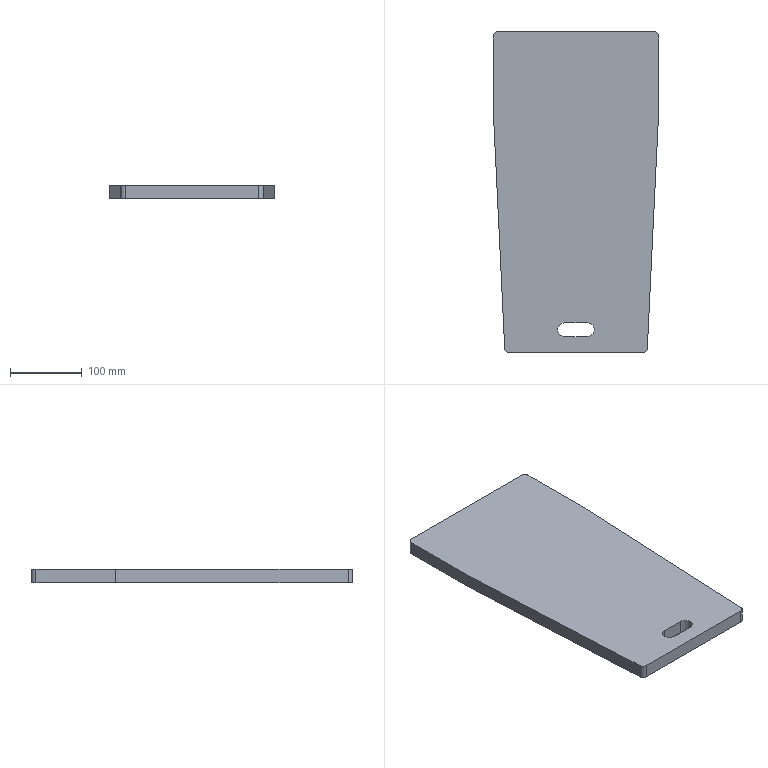Part | SolidWorks | features Extrusion 1 | 1 solid | 17 faces | box 230 x 447.55 x 19.05 mm | volume 1843027 mm3 | plane 10 | cylinder 7 | commonest cylinder face diameters 12.7 x4 19.05 x3
STEP:
#1=CARTESIAN_POINT('',(-15.875,9.525,9.525));
#2=VERTEX_POINT('',#1);
#3=CARTESIAN_POINT('',(-25.4,0.,9.525));
#4=VERTEX_POINT('',#3);
#5=CARTESIAN_POINT('',(-15.875,0.,9.525));
#6=DIRECTION('',(0.,0.,1.));
#7=DIRECTION('',(1.,0.,0.));
#8=AXIS2_PLACEMENT_3D('',#5,#6,#7);
#9=CIRCLE('',#8,9.525);
#10=EDGE_CURVE('',#2,#4,#9,.T.);
#11=ORIENTED_EDGE('',*,*,#10,.T.);
#12=CARTESIAN_POINT('',(-25.4,0.,-9.525));
#13=VERTEX_POINT('',#12);
#14=CARTESIAN_POINT('',(-25.4,0.,9.525));
#15=DIRECTION('',(0.,0.,-1.));
#16=VECTOR('',#15,1000.);
#17=LINE('',#14,#16);
#18=EDGE_CURVE('',#4,#13,#17,.T.);
#19=ORIENTED_EDGE('',*,*,#18,.T.);
#20=CARTESIAN_POINT('',(-15.875,9.525,-9.525));
#21=VERTEX_POINT('',#20);
#22=CARTESIAN_POINT('',(-15.875,0.,-9.525));
#23=DIRECTION('',(0.,0.,1.));
#24=DIRECTION('',(1.,0.,0.));
#25=AXIS2_PLACEMENT_3D('',#22,#23,#24);
#26=CIRCLE('',#25,9.525);
#27=EDGE_CURVE('',#21,#13,#26,.T.);
#28=ORIENTED_EDGE('',*,*,#27,.F.);
#29=CARTESIAN_POINT('',(-15.875,9.525,9.525));
#30=DIRECTION('',(0.,0.,-1.));
#31=VECTOR('',#30,1000.);
#32=LINE('',#29,#31);
#33=EDGE_CURVE('',#2,#21,#32,.T.);
#34=ORIENTED_EDGE('',*,*,#33,.F.);
#35=EDGE_LOOP('',(#11,#19,#28,#34));
#36=FACE_OUTER_BOUND('',#35,.T.);
#37=CARTESIAN_POINT('',(-15.875,0.,9.525));
#38=DIRECTION('',(0.,0.,-1.));
#39=DIRECTION('',(-1.,0.,0.));
#40=AXIS2_PLACEMENT_3D('',#37,#38,#39);
#41=CYLINDRICAL_SURFACE('',#40,9.525);
#42=ADVANCED_FACE('',(#36),#41,.F.);
#43=CARTESIAN_POINT('',(-115.,298.68,9.525));
#44=VERTEX_POINT('',#43);
#45=CARTESIAN_POINT('',(-99.352,-25.706,9.525));
#46=VERTEX_POINT('',#45);
#47=CARTESIAN_POINT('',(-115.,298.68,9.525));
#48=DIRECTION('',(0.04818,-0.9988,0.));
#49=VECTOR('',#48,1000.);
#50=LINE('',#47,#49);
#51=EDGE_CURVE('',#44,#46,#50,.T.);
#52=ORIENTED_EDGE('',*,*,#51,.T.);
#53=CARTESIAN_POINT('',(-93.009,-31.75,9.525));
#54=VERTEX_POINT('',#53);
#55=CARTESIAN_POINT('',(-93.009,-25.4,9.525));
#56=DIRECTION('',(0.,0.,1.));
#57=DIRECTION('',(1.,0.,0.));
#58=AXIS2_PLACEMENT_3D('',#55,#56,#57);
#59=CIRCLE('',#58,6.35);
#60=EDGE_CURVE('',#46,#54,#59,.T.);
#61=ORIENTED_EDGE('',*,*,#60,.T.);
#62=CARTESIAN_POINT('',(93.009,-31.75,9.525));
#63=VERTEX_POINT('',#62);
#64=CARTESIAN_POINT('',(-93.009,-31.75,9.525));
#65=DIRECTION('',(1.,0.,0.));
#66=VECTOR('',#65,1000.);
#67=LINE('',#64,#66);
#68=EDGE_CURVE('',#54,#63,#67,.T.);
#69=ORIENTED_EDGE('',*,*,#68,.T.);
#70=CARTESIAN_POINT('',(99.352,-25.706,9.525));
#71=VERTEX_POINT('',#70);
#72=CARTESIAN_POINT('',(93.009,-25.4,9.525));
#73=DIRECTION('',(0.,0.,1.));
#74=DIRECTION('',(-1.,0.,0.));
#75=AXIS2_PLACEMENT_3D('',#72,#73,#74);
#76=CIRCLE('',#75,6.35);
#77=EDGE_CURVE('',#63,#71,#76,.T.);
#78=ORIENTED_EDGE('',*,*,#77,.T.);
#79=CARTESIAN_POINT('',(115.,298.68,9.525));
#80=VERTEX_POINT('',#79);
#81=CARTESIAN_POINT('',(115.,298.68,9.525));
#82=DIRECTION('',(0.04818,0.9988,0.));
#83=VECTOR('',#82,1000.);
#84=LINE('',#81,#83);
#85=EDGE_CURVE('',#71,#80,#84,.T.);
#86=ORIENTED_EDGE('',*,*,#85,.T.);
#87=CARTESIAN_POINT('',(115.,409.45,9.525));
#88=VERTEX_POINT('',#87);
#89=CARTESIAN_POINT('',(115.,409.45,9.525));
#90=DIRECTION('',(0.,1.,0.));
#91=VECTOR('',#90,1000.);
#92=LINE('',#89,#91);
#93=EDGE_CURVE('',#80,#88,#92,.T.);
#94=ORIENTED_EDGE('',*,*,#93,.T.);
#95=CARTESIAN_POINT('',(108.65,415.8,9.525));
#96=VERTEX_POINT('',#95);
#97=CARTESIAN_POINT('',(108.65,409.45,9.525));
#98=DIRECTION('',(0.,0.,1.));
#99=DIRECTION('',(-1.,0.,0.));
#100=AXIS2_PLACEMENT_3D('',#97,#98,#99);
#101=CIRCLE('',#100,6.35);
#102=EDGE_CURVE('',#88,#96,#101,.T.);
#103=ORIENTED_EDGE('',*,*,#102,.T.);
#104=CARTESIAN_POINT('',(-108.65,415.8,9.525));
#105=VERTEX_POINT('',#104);
#106=CARTESIAN_POINT('',(108.65,415.8,9.525));
#107=DIRECTION('',(-1.,0.,0.));
#108=VECTOR('',#107,1000.);
#109=LINE('',#106,#108);
#110=EDGE_CURVE('',#96,#105,#109,.T.);
#111=ORIENTED_EDGE('',*,*,#110,.T.);
#112=CARTESIAN_POINT('',(-115.,409.45,9.525));
#113=VERTEX_POINT('',#112);
#114=CARTESIAN_POINT('',(-108.65,409.45,9.525));
#115=DIRECTION('',(0.,0.,1.));
#116=DIRECTION('',(1.,0.,0.));
#117=AXIS2_PLACEMENT_3D('',#114,#115,#116);
#118=CIRCLE('',#117,6.35);
#119=EDGE_CURVE('',#105,#113,#118,.T.);
#120=ORIENTED_EDGE('',*,*,#119,.T.);
#121=CARTESIAN_POINT('',(-115.,409.45,9.525));
#122=DIRECTION('',(0.,-1.,0.));
#123=VECTOR('',#122,1000.);
#124=LINE('',#121,#123);
#125=EDGE_CURVE('',#113,#44,#124,.T.);
#126=ORIENTED_EDGE('',*,*,#125,.T.);
#127=EDGE_LOOP('',(#52,#61,#69,#78,#86,#94,#103,#111,#120,#126));
#128=FACE_OUTER_BOUND('',#127,.T.);
#129=CARTESIAN_POINT('',(-15.875,-9.525,9.525));
#130=VERTEX_POINT('',#129);
#131=CARTESIAN_POINT('',(15.875,-9.525,9.525));
#132=VERTEX_POINT('',#131);
#133=CARTESIAN_POINT('',(-15.875,-9.525,9.525));
#134=DIRECTION('',(1.,0.,0.));
#135=VECTOR('',#134,1000.);
#136=LINE('',#133,#135);
#137=EDGE_CURVE('',#130,#132,#136,.T.);
#138=ORIENTED_EDGE('',*,*,#137,.F.);
#139=CARTESIAN_POINT('',(-15.875,0.,9.525));
#140=DIRECTION('',(0.,0.,1.));
#141=DIRECTION('',(1.,0.,0.));
#142=AXIS2_PLACEMENT_3D('',#139,#140,#141);
#143=CIRCLE('',#142,9.525);
#144=EDGE_CURVE('',#4,#130,#143,.T.);
#145=ORIENTED_EDGE('',*,*,#144,.F.);
#146=ORIENTED_EDGE('',*,*,#10,.F.);
#147=CARTESIAN_POINT('',(15.875,9.525,9.525));
#148=VERTEX_POINT('',#147);
#149=CARTESIAN_POINT('',(-15.875,9.525,9.525));
#150=DIRECTION('',(-1.,0.,0.));
#151=VECTOR('',#150,1000.);
#152=LINE('',#149,#151);
#153=EDGE_CURVE('',#148,#2,#152,.T.);
#154=ORIENTED_EDGE('',*,*,#153,.F.);
#155=CARTESIAN_POINT('',(15.875,0.,9.525));
#156=DIRECTION('',(0.,0.,1.));
#157=DIRECTION('',(1.,0.,0.));
#158=AXIS2_PLACEMENT_3D('',#155,#156,#157);
#159=CIRCLE('',#158,9.525);
#160=EDGE_CURVE('',#132,#148,#159,.T.);
#161=ORIENTED_EDGE('',*,*,#160,.F.);
#162=EDGE_LOOP('',(#138,#145,#146,#154,#161));
#163=FACE_BOUND('',#162,.T.);
#164=CARTESIAN_POINT('',(-93.009,-25.4,9.525));
#165=DIRECTION('',(0.,0.,1.));
#166=DIRECTION('',(1.,0.,0.));
#167=AXIS2_PLACEMENT_3D('',#164,#165,#166);
#168=PLANE('',#167);
#169=ADVANCED_FACE('',(#128,#163),#168,.T.);
#170=CARTESIAN_POINT('',(-115.,298.68,-9.525));
#171=VERTEX_POINT('',#170);
#172=CARTESIAN_POINT('',(-99.352,-25.706,-9.525));
#173=VERTEX_POINT('',#172);
#174=CARTESIAN_POINT('',(-115.,298.68,-9.525));
#175=DIRECTION('',(0.04818,-0.9988,0.));
#176=VECTOR('',#175,1000.);
#177=LINE('',#174,#176);
#178=EDGE_CURVE('',#171,#173,#177,.T.);
#179=ORIENTED_EDGE('',*,*,#178,.F.);
#180=CARTESIAN_POINT('',(-115.,409.45,-9.525));
#181=VERTEX_POINT('',#180);
#182=CARTESIAN_POINT('',(-115.,409.45,-9.525));
#183=DIRECTION('',(0.,-1.,0.));
#184=VECTOR('',#183,1000.);
#185=LINE('',#182,#184);
#186=EDGE_CURVE('',#181,#171,#185,.T.);
#187=ORIENTED_EDGE('',*,*,#186,.F.);
#188=CARTESIAN_POINT('',(-108.65,415.8,-9.525));
#189=VERTEX_POINT('',#188);
#190=CARTESIAN_POINT('',(-108.65,409.45,-9.525));
#191=DIRECTION('',(0.,0.,1.));
#192=DIRECTION('',(1.,0.,0.));
#193=AXIS2_PLACEMENT_3D('',#190,#191,#192);
#194=CIRCLE('',#193,6.35);
#195=EDGE_CURVE('',#189,#181,#194,.T.);
#196=ORIENTED_EDGE('',*,*,#195,.F.);
#197=CARTESIAN_POINT('',(108.65,415.8,-9.525));
#198=VERTEX_POINT('',#197);
#199=CARTESIAN_POINT('',(108.65,415.8,-9.525));
#200=DIRECTION('',(-1.,0.,0.));
#201=VECTOR('',#200,1000.);
#202=LINE('',#199,#201);
#203=EDGE_CURVE('',#198,#189,#202,.T.);
#204=ORIENTED_EDGE('',*,*,#203,.F.);
#205=CARTESIAN_POINT('',(115.,409.45,-9.525));
#206=VERTEX_POINT('',#205);
#207=CARTESIAN_POINT('',(108.65,409.45,-9.525));
#208=DIRECTION('',(0.,0.,1.));
#209=DIRECTION('',(-1.,0.,0.));
#210=AXIS2_PLACEMENT_3D('',#207,#208,#209);
#211=CIRCLE('',#210,6.35);
#212=EDGE_CURVE('',#206,#198,#211,.T.);
#213=ORIENTED_EDGE('',*,*,#212,.F.);
#214=CARTESIAN_POINT('',(115.,298.68,-9.525));
#215=VERTEX_POINT('',#214);
#216=CARTESIAN_POINT('',(115.,409.45,-9.525));
#217=DIRECTION('',(0.,1.,0.));
#218=VECTOR('',#217,1000.);
#219=LINE('',#216,#218);
#220=EDGE_CURVE('',#215,#206,#219,.T.);
#221=ORIENTED_EDGE('',*,*,#220,.F.);
#222=CARTESIAN_POINT('',(99.352,-25.706,-9.525));
#223=VERTEX_POINT('',#222);
#224=CARTESIAN_POINT('',(115.,298.68,-9.525));
#225=DIRECTION('',(0.04818,0.9988,0.));
#226=VECTOR('',#225,1000.);
#227=LINE('',#224,#226);
#228=EDGE_CURVE('',#223,#215,#227,.T.);
#229=ORIENTED_EDGE('',*,*,#228,.F.);
#230=CARTESIAN_POINT('',(93.009,-31.75,-9.525));
#231=VERTEX_POINT('',#230);
#232=CARTESIAN_POINT('',(93.009,-25.4,-9.525));
#233=DIRECTION('',(0.,0.,1.));
#234=DIRECTION('',(-1.,0.,0.));
#235=AXIS2_PLACEMENT_3D('',#232,#233,#234);
#236=CIRCLE('',#235,6.35);
#237=EDGE_CURVE('',#231,#223,#236,.T.);
#238=ORIENTED_EDGE('',*,*,#237,.F.);
#239=CARTESIAN_POINT('',(-93.009,-31.75,-9.525));
#240=VERTEX_POINT('',#239);
#241=CARTESIAN_POINT('',(-93.009,-31.75,-9.525));
#242=DIRECTION('',(1.,0.,0.));
#243=VECTOR('',#242,1000.);
#244=LINE('',#241,#243);
#245=EDGE_CURVE('',#240,#231,#244,.T.);
#246=ORIENTED_EDGE('',*,*,#245,.F.);
#247=CARTESIAN_POINT('',(-93.009,-25.4,-9.525));
#248=DIRECTION('',(0.,0.,1.));
#249=DIRECTION('',(1.,0.,0.));
#250=AXIS2_PLACEMENT_3D('',#247,#248,#249);
#251=CIRCLE('',#250,6.35);
#252=EDGE_CURVE('',#173,#240,#251,.T.);
#253=ORIENTED_EDGE('',*,*,#252,.F.);
#254=EDGE_LOOP('',(#179,#187,#196,#204,#213,#221,#229,#238,#246,#253));
#255=FACE_OUTER_BOUND('',#254,.T.);
#256=ORIENTED_EDGE('',*,*,#27,.T.);
#257=CARTESIAN_POINT('',(-15.875,-9.525,-9.525));
#258=VERTEX_POINT('',#257);
#259=CARTESIAN_POINT('',(-15.875,0.,-9.525));
#260=DIRECTION('',(0.,0.,1.));
#261=DIRECTION('',(1.,0.,0.));
#262=AXIS2_PLACEMENT_3D('',#259,#260,#261);
#263=CIRCLE('',#262,9.525);
#264=EDGE_CURVE('',#13,#258,#263,.T.);
#265=ORIENTED_EDGE('',*,*,#264,.T.);
#266=CARTESIAN_POINT('',(15.875,-9.525,-9.525));
#267=VERTEX_POINT('',#266);
#268=CARTESIAN_POINT('',(-15.875,-9.525,-9.525));
#269=DIRECTION('',(1.,0.,0.));
#270=VECTOR('',#269,1000.);
#271=LINE('',#268,#270);
#272=EDGE_CURVE('',#258,#267,#271,.T.);
#273=ORIENTED_EDGE('',*,*,#272,.T.);
#274=CARTESIAN_POINT('',(15.875,9.525,-9.525));
#275=VERTEX_POINT('',#274);
#276=CARTESIAN_POINT('',(15.875,0.,-9.525));
#277=DIRECTION('',(0.,0.,1.));
#278=DIRECTION('',(1.,0.,0.));
#279=AXIS2_PLACEMENT_3D('',#276,#277,#278);
#280=CIRCLE('',#279,9.525);
#281=EDGE_CURVE('',#267,#275,#280,.T.);
#282=ORIENTED_EDGE('',*,*,#281,.T.);
#283=CARTESIAN_POINT('',(-15.875,9.525,-9.525));
#284=DIRECTION('',(-1.,0.,0.));
#285=VECTOR('',#284,1000.);
#286=LINE('',#283,#285);
#287=EDGE_CURVE('',#275,#21,#286,.T.);
#288=ORIENTED_EDGE('',*,*,#287,.T.);
#289=EDGE_LOOP('',(#256,#265,#273,#282,#288));
#290=FACE_BOUND('',#289,.T.);
#291=CARTESIAN_POINT('',(-93.009,-25.4,-9.525));
#292=DIRECTION('',(0.,0.,1.));
#293=DIRECTION('',(1.,0.,0.));
#294=AXIS2_PLACEMENT_3D('',#291,#292,#293);
#295=PLANE('',#294);
#296=ADVANCED_FACE('',(#255,#290),#295,.F.);
#297=ORIENTED_EDGE('',*,*,#178,.T.);
#298=CARTESIAN_POINT('',(-99.352,-25.706,9.525));
#299=DIRECTION('',(0.,0.,-1.));
#300=VECTOR('',#299,1000.);
#301=LINE('',#298,#300);
#302=EDGE_CURVE('',#46,#173,#301,.T.);
#303=ORIENTED_EDGE('',*,*,#302,.F.);
#304=ORIENTED_EDGE('',*,*,#51,.F.);
#305=CARTESIAN_POINT('',(-115.,298.68,9.525));
#306=DIRECTION('',(0.,0.,-1.));
#307=VECTOR('',#306,1000.);
#308=LINE('',#305,#307);
#309=EDGE_CURVE('',#44,#171,#308,.T.);
#310=ORIENTED_EDGE('',*,*,#309,.T.);
#311=EDGE_LOOP('',(#297,#303,#304,#310));
#312=FACE_OUTER_BOUND('',#311,.T.);
#313=CARTESIAN_POINT('',(-115.,298.68,9.525));
#314=DIRECTION('',(0.9988,0.04818,0.));
#315=DIRECTION('',(-0.04818,0.9988,0.));
#316=AXIS2_PLACEMENT_3D('',#313,#314,#315);
#317=PLANE('',#316);
#318=ADVANCED_FACE('',(#312),#317,.F.);
#319=ORIENTED_EDGE('',*,*,#252,.T.);
#320=CARTESIAN_POINT('',(-93.009,-31.75,9.525));
#321=DIRECTION('',(0.,0.,-1.));
#322=VECTOR('',#321,1000.);
#323=LINE('',#320,#322);
#324=EDGE_CURVE('',#54,#240,#323,.T.);
#325=ORIENTED_EDGE('',*,*,#324,.F.);
#326=ORIENTED_EDGE('',*,*,#60,.F.);
#327=ORIENTED_EDGE('',*,*,#302,.T.);
#328=EDGE_LOOP('',(#319,#325,#326,#327));
#329=FACE_OUTER_BOUND('',#328,.T.);
#330=CARTESIAN_POINT('',(-93.009,-25.4,9.525));
#331=DIRECTION('',(0.,0.,-1.));
#332=DIRECTION('',(-1.,0.,0.));
#333=AXIS2_PLACEMENT_3D('',#330,#331,#332);
#334=CYLINDRICAL_SURFACE('',#333,6.35);
#335=ADVANCED_FACE('',(#329),#334,.T.);
#336=ORIENTED_EDGE('',*,*,#245,.T.);
#337=CARTESIAN_POINT('',(93.009,-31.75,9.525));
#338=DIRECTION('',(0.,0.,-1.));
#339=VECTOR('',#338,1000.);
#340=LINE('',#337,#339);
#341=EDGE_CURVE('',#63,#231,#340,.T.);
#342=ORIENTED_EDGE('',*,*,#341,.F.);
#343=ORIENTED_EDGE('',*,*,#68,.F.);
#344=ORIENTED_EDGE('',*,*,#324,.T.);
#345=EDGE_LOOP('',(#336,#342,#343,#344));
#346=FACE_OUTER_BOUND('',#345,.T.);
#347=CARTESIAN_POINT('',(-93.009,-31.75,9.525));
#348=DIRECTION('',(0.,1.,0.));
#349=DIRECTION('',(0.,0.,1.));
#350=AXIS2_PLACEMENT_3D('',#347,#348,#349);
#351=PLANE('',#350);
#352=ADVANCED_FACE('',(#346),#351,.F.);
#353=ORIENTED_EDGE('',*,*,#237,.T.);
#354=CARTESIAN_POINT('',(99.352,-25.706,9.525));
#355=DIRECTION('',(0.,0.,-1.));
#356=VECTOR('',#355,1000.);
#357=LINE('',#354,#356);
#358=EDGE_CURVE('',#71,#223,#357,.T.);
#359=ORIENTED_EDGE('',*,*,#358,.F.);
#360=ORIENTED_EDGE('',*,*,#77,.F.);
#361=ORIENTED_EDGE('',*,*,#341,.T.);
#362=EDGE_LOOP('',(#353,#359,#360,#361));
#363=FACE_OUTER_BOUND('',#362,.T.);
#364=CARTESIAN_POINT('',(93.009,-25.4,9.525));
#365=DIRECTION('',(0.,0.,-1.));
#366=DIRECTION('',(-1.,0.,0.));
#367=AXIS2_PLACEMENT_3D('',#364,#365,#366);
#368=CYLINDRICAL_SURFACE('',#367,6.35);
#369=ADVANCED_FACE('',(#363),#368,.T.);
#370=ORIENTED_EDGE('',*,*,#228,.T.);
#371=CARTESIAN_POINT('',(115.,298.68,9.525));
#372=DIRECTION('',(0.,0.,-1.));
#373=VECTOR('',#372,1000.);
#374=LINE('',#371,#373);
#375=EDGE_CURVE('',#80,#215,#374,.T.);
#376=ORIENTED_EDGE('',*,*,#375,.F.);
#377=ORIENTED_EDGE('',*,*,#85,.F.);
#378=ORIENTED_EDGE('',*,*,#358,.T.);
#379=EDGE_LOOP('',(#370,#376,#377,#378));
#380=FACE_OUTER_BOUND('',#379,.T.);
#381=CARTESIAN_POINT('',(115.,298.68,9.525));
#382=DIRECTION('',(-0.9988,0.04818,0.));
#383=DIRECTION('',(-0.04818,-0.9988,0.));
#384=AXIS2_PLACEMENT_3D('',#381,#382,#383);
#385=PLANE('',#384);
#386=ADVANCED_FACE('',(#380),#385,.F.);
#387=ORIENTED_EDGE('',*,*,#220,.T.);
#388=CARTESIAN_POINT('',(115.,409.45,9.525));
#389=DIRECTION('',(0.,0.,-1.));
#390=VECTOR('',#389,1000.);
#391=LINE('',#388,#390);
#392=EDGE_CURVE('',#88,#206,#391,.T.);
#393=ORIENTED_EDGE('',*,*,#392,.F.);
#394=ORIENTED_EDGE('',*,*,#93,.F.);
#395=ORIENTED_EDGE('',*,*,#375,.T.);
#396=EDGE_LOOP('',(#387,#393,#394,#395));
#397=FACE_OUTER_BOUND('',#396,.T.);
#398=CARTESIAN_POINT('',(115.,409.45,9.525));
#399=DIRECTION('',(-1.,0.,0.));
#400=DIRECTION('',(0.,0.,1.));
#401=AXIS2_PLACEMENT_3D('',#398,#399,#400);
#402=PLANE('',#401);
#403=ADVANCED_FACE('',(#397),#402,.F.);
#404=ORIENTED_EDGE('',*,*,#212,.T.);
#405=CARTESIAN_POINT('',(108.65,415.8,9.525));
#406=DIRECTION('',(0.,0.,-1.));
#407=VECTOR('',#406,1000.);
#408=LINE('',#405,#407);
#409=EDGE_CURVE('',#96,#198,#408,.T.);
#410=ORIENTED_EDGE('',*,*,#409,.F.);
#411=ORIENTED_EDGE('',*,*,#102,.F.);
#412=ORIENTED_EDGE('',*,*,#392,.T.);
#413=EDGE_LOOP('',(#404,#410,#411,#412));
#414=FACE_OUTER_BOUND('',#413,.T.);
#415=CARTESIAN_POINT('',(108.65,409.45,9.525));
#416=DIRECTION('',(0.,0.,-1.));
#417=DIRECTION('',(-1.,0.,0.));
#418=AXIS2_PLACEMENT_3D('',#415,#416,#417);
#419=CYLINDRICAL_SURFACE('',#418,6.35);
#420=ADVANCED_FACE('',(#414),#419,.T.);
#421=ORIENTED_EDGE('',*,*,#203,.T.);
#422=CARTESIAN_POINT('',(-108.65,415.8,9.525));
#423=DIRECTION('',(0.,0.,-1.));
#424=VECTOR('',#423,1000.);
#425=LINE('',#422,#424);
#426=EDGE_CURVE('',#105,#189,#425,.T.);
#427=ORIENTED_EDGE('',*,*,#426,.F.);
#428=ORIENTED_EDGE('',*,*,#110,.F.);
#429=ORIENTED_EDGE('',*,*,#409,.T.);
#430=EDGE_LOOP('',(#421,#427,#428,#429));
#431=FACE_OUTER_BOUND('',#430,.T.);
#432=CARTESIAN_POINT('',(108.65,415.8,9.525));
#433=DIRECTION('',(0.,-1.,0.));
#434=DIRECTION('',(0.,0.,-1.));
#435=AXIS2_PLACEMENT_3D('',#432,#433,#434);
#436=PLANE('',#435);
#437=ADVANCED_FACE('',(#431),#436,.F.);
#438=ORIENTED_EDGE('',*,*,#195,.T.);
#439=CARTESIAN_POINT('',(-115.,409.45,9.525));
#440=DIRECTION('',(0.,0.,-1.));
#441=VECTOR('',#440,1000.);
#442=LINE('',#439,#441);
#443=EDGE_CURVE('',#113,#181,#442,.T.);
#444=ORIENTED_EDGE('',*,*,#443,.F.);
#445=ORIENTED_EDGE('',*,*,#119,.F.);
#446=ORIENTED_EDGE('',*,*,#426,.T.);
#447=EDGE_LOOP('',(#438,#444,#445,#446));
#448=FACE_OUTER_BOUND('',#447,.T.);
#449=CARTESIAN_POINT('',(-108.65,409.45,9.525));
#450=DIRECTION('',(0.,0.,-1.));
#451=DIRECTION('',(-1.,0.,0.));
#452=AXIS2_PLACEMENT_3D('',#449,#450,#451);
#453=CYLINDRICAL_SURFACE('',#452,6.35);
#454=ADVANCED_FACE('',(#448),#453,.T.);
#455=ORIENTED_EDGE('',*,*,#186,.T.);
#456=ORIENTED_EDGE('',*,*,#309,.F.);
#457=ORIENTED_EDGE('',*,*,#125,.F.);
#458=ORIENTED_EDGE('',*,*,#443,.T.);
#459=EDGE_LOOP('',(#455,#456,#457,#458));
#460=FACE_OUTER_BOUND('',#459,.T.);
#461=CARTESIAN_POINT('',(-115.,409.45,9.525));
#462=DIRECTION('',(1.,0.,0.));
#463=DIRECTION('',(0.,0.,-1.));
#464=AXIS2_PLACEMENT_3D('',#461,#462,#463);
#465=PLANE('',#464);
#466=ADVANCED_FACE('',(#460),#465,.F.);
#467=ORIENTED_EDGE('',*,*,#18,.F.);
#468=ORIENTED_EDGE('',*,*,#144,.T.);
#469=CARTESIAN_POINT('',(-15.875,-9.525,9.525));
#470=DIRECTION('',(0.,0.,-1.));
#471=VECTOR('',#470,1000.);
#472=LINE('',#469,#471);
#473=EDGE_CURVE('',#130,#258,#472,.T.);
#474=ORIENTED_EDGE('',*,*,#473,.T.);
#475=ORIENTED_EDGE('',*,*,#264,.F.);
#476=EDGE_LOOP('',(#467,#468,#474,#475));
#477=FACE_OUTER_BOUND('',#476,.T.);
#478=CARTESIAN_POINT('',(-15.875,0.,9.525));
#479=DIRECTION('',(0.,0.,-1.));
#480=DIRECTION('',(-1.,0.,0.));
#481=AXIS2_PLACEMENT_3D('',#478,#479,#480);
#482=CYLINDRICAL_SURFACE('',#481,9.525);
#483=ADVANCED_FACE('',(#477),#482,.F.);
#484=ORIENTED_EDGE('',*,*,#272,.F.);
#485=ORIENTED_EDGE('',*,*,#473,.F.);
#486=ORIENTED_EDGE('',*,*,#137,.T.);
#487=CARTESIAN_POINT('',(15.875,-9.525,9.525));
#488=DIRECTION('',(0.,0.,-1.));
#489=VECTOR('',#488,1000.);
#490=LINE('',#487,#489);
#491=EDGE_CURVE('',#132,#267,#490,.T.);
#492=ORIENTED_EDGE('',*,*,#491,.T.);
#493=EDGE_LOOP('',(#484,#485,#486,#492));
#494=FACE_OUTER_BOUND('',#493,.T.);
#495=CARTESIAN_POINT('',(-15.875,-9.525,9.525));
#496=DIRECTION('',(0.,1.,0.));
#497=DIRECTION('',(-1.,0.,0.));
#498=AXIS2_PLACEMENT_3D('',#495,#496,#497);
#499=PLANE('',#498);
#500=ADVANCED_FACE('',(#494),#499,.T.);
#501=ORIENTED_EDGE('',*,*,#281,.F.);
#502=ORIENTED_EDGE('',*,*,#491,.F.);
#503=ORIENTED_EDGE('',*,*,#160,.T.);
#504=CARTESIAN_POINT('',(15.875,9.525,9.525));
#505=DIRECTION('',(0.,0.,-1.));
#506=VECTOR('',#505,1000.);
#507=LINE('',#504,#506);
#508=EDGE_CURVE('',#148,#275,#507,.T.);
#509=ORIENTED_EDGE('',*,*,#508,.T.);
#510=EDGE_LOOP('',(#501,#502,#503,#509));
#511=FACE_OUTER_BOUND('',#510,.T.);
#512=CARTESIAN_POINT('',(15.875,0.,9.525));
#513=DIRECTION('',(0.,0.,-1.));
#514=DIRECTION('',(-1.,0.,0.));
#515=AXIS2_PLACEMENT_3D('',#512,#513,#514);
#516=CYLINDRICAL_SURFACE('',#515,9.525);
#517=ADVANCED_FACE('',(#511),#516,.F.);
#518=ORIENTED_EDGE('',*,*,#287,.F.);
#519=ORIENTED_EDGE('',*,*,#508,.F.);
#520=ORIENTED_EDGE('',*,*,#153,.T.);
#521=ORIENTED_EDGE('',*,*,#33,.T.);
#522=EDGE_LOOP('',(#518,#519,#520,#521));
#523=FACE_OUTER_BOUND('',#522,.T.);
#524=CARTESIAN_POINT('',(-15.875,9.525,9.525));
#525=DIRECTION('',(0.,-1.,0.));
#526=DIRECTION('',(1.,0.,0.));
#527=AXIS2_PLACEMENT_3D('',#524,#525,#526);
#528=PLANE('',#527);
#529=ADVANCED_FACE('',(#523),#528,.T.);
#530=CLOSED_SHELL('',(#42,#169,#296,#318,#335,#352,#369,#386,#403,#420,#437,#454,#466,#483,#500,#517,#529));
#531=MANIFOLD_SOLID_BREP('',#530);
#532=CARTESIAN_POINT('',(0.,0.,0.));
#533=DIRECTION('',(0.,0.,1.));
#534=DIRECTION('',(1.,0.,0.));
#535=AXIS2_PLACEMENT_3D('',#532,#533,#534);
#536=(LENGTH_UNIT()NAMED_UNIT(*)SI_UNIT(.MILLI.,.METRE.));
#537=UNCERTAINTY_MEASURE_WITH_UNIT(LENGTH_MEASURE(0.00001),#536,'','');
#538=(NAMED_UNIT(*)PLANE_ANGLE_UNIT()SI_UNIT($,.RADIAN.));
#539=(NAMED_UNIT(*)SI_UNIT($,.STERADIAN.)SOLID_ANGLE_UNIT());
#540=(GEOMETRIC_REPRESENTATION_CONTEXT(3)GLOBAL_UNCERTAINTY_ASSIGNED_CONTEXT((#537))GLOBAL_UNIT_ASSIGNED_CONTEXT((#536,#538,#539))REPRESENTATION_CONTEXT('',''));
#541=ADVANCED_BREP_SHAPE_REPRESENTATION('',(#531,#535),#540);